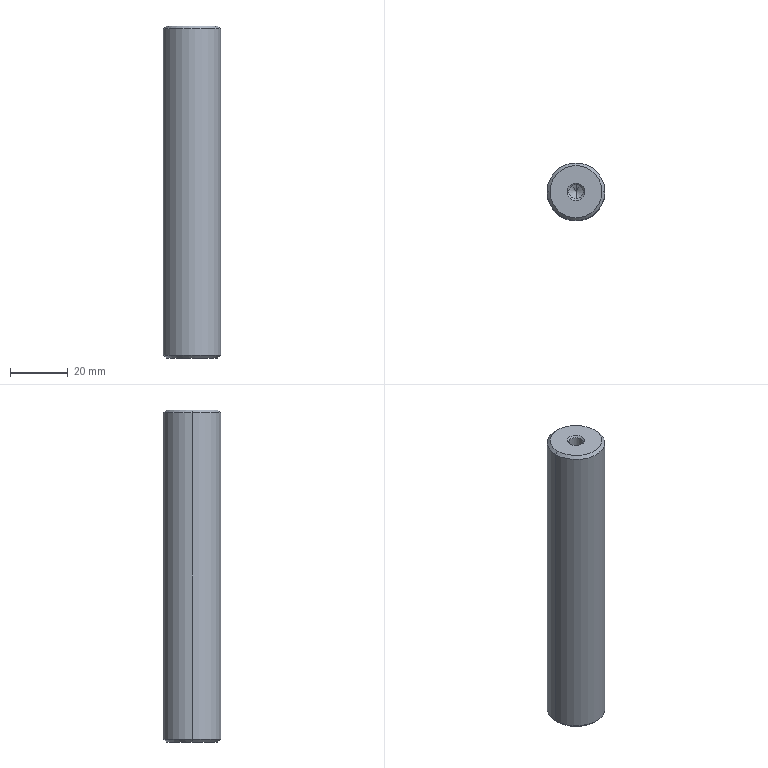Part | STEP file | 001-011-SCD21-D20-L115-M6 | 1 solid | 14 faces | box 20 x 20 x 115 mm | volume 35828 mm3 | cone 8 | cylinder 4 | plane 2 | commonest cylinder face diameters 4.917 x2 20 x2
STEP:
#1=CARTESIAN_POINT('',(0.,0.,0.));
#2=DIRECTION('',(0.,0.,1.));
#3=DIRECTION('',(1.,0.,0.));
#4=AXIS2_PLACEMENT_3D('',#1,#2,#3);
#5=CARTESIAN_POINT('',(0.,-2.458,-12.));
#6=VERTEX_POINT('',#5);
#7=CARTESIAN_POINT('',(0.,2.458,-12.));
#8=VERTEX_POINT('',#7);
#9=CARTESIAN_POINT('',(0.,0.,-12.));
#10=DIRECTION('',(0.,0.,-1.));
#11=DIRECTION('',(0.,1.,0.));
#12=AXIS2_PLACEMENT_3D('',#9,#10,#11);
#13=CIRCLE('',#12,2.458);
#14=CARTESIAN_POINT('',(0.,0.,-12.));
#15=DIRECTION('',(0.,0.,1.));
#16=DIRECTION('',(0.,-1.,0.));
#17=AXIS2_PLACEMENT_3D('',#14,#15,#16);
#18=CONICAL_SURFACE('',#17,2.458,1.047);
#19=CARTESIAN_POINT('',(9.425,0.));
#20=DIRECTION('',(-1.,0.));
#21=VECTOR('',#20,1.);
#22=LINE('',#19,#21);
#23=(GEOMETRIC_REPRESENTATION_CONTEXT(2)PARAMETRIC_REPRESENTATION_CONTEXT()REPRESENTATION_CONTEXT('',''));
#24=DEFINITIONAL_REPRESENTATION('',(#22),#23);
#25=PCURVE('',#18,#24);
#26=CARTESIAN_POINT('',(0.,0.,-13.419));
#27=DIRECTION('',(0.,0.,1.));
#28=DIRECTION('',(0.,1.,0.));
#29=AXIS2_PLACEMENT_3D('',#26,#27,#28);
#30=CYLINDRICAL_SURFACE('',#29,2.458);
#31=CARTESIAN_POINT('',(6.283,1.419));
#32=DIRECTION('',(-1.,0.));
#33=VECTOR('',#32,1.);
#34=LINE('',#31,#33);
#35=(GEOMETRIC_REPRESENTATION_CONTEXT(2)PARAMETRIC_REPRESENTATION_CONTEXT()REPRESENTATION_CONTEXT('',''));
#36=DEFINITIONAL_REPRESENTATION('',(#34),#35);
#37=PCURVE('',#30,#36);
#38=SURFACE_CURVE('',#13,(#25,#37),.PCURVE_S1.);
#39=EDGE_CURVE('',#6,#8,#38,.T.);
#40=ORIENTED_EDGE('',*,*,#39,.T.);
#41=CARTESIAN_POINT('',(0.,0.,-13.419));
#42=VERTEX_POINT('',#41);
#43=CARTESIAN_POINT('',(0.,2.458,-12.));
#44=DIRECTION('',(0.,0.866,0.5));
#45=VECTOR('',#44,1.);
#46=LINE('',#43,#45);
#47=CARTESIAN_POINT('',(3.142,0.));
#48=DIRECTION('',(0.,1.));
#49=VECTOR('',#48,1.);
#50=LINE('',#47,#49);
#51=(GEOMETRIC_REPRESENTATION_CONTEXT(2)PARAMETRIC_REPRESENTATION_CONTEXT()REPRESENTATION_CONTEXT('',''));
#52=DEFINITIONAL_REPRESENTATION('',(#50),#51);
#53=PCURVE('',#18,#52);
#54=CARTESIAN_POINT('',(0.,0.,-12.));
#55=DIRECTION('',(0.,0.,1.));
#56=DIRECTION('',(0.,-1.,0.));
#57=AXIS2_PLACEMENT_3D('',#54,#55,#56);
#58=CONICAL_SURFACE('',#57,2.458,1.047);
#59=CARTESIAN_POINT('',(3.142,0.));
#60=DIRECTION('',(0.,1.));
#61=VECTOR('',#60,1.);
#62=LINE('',#59,#61);
#63=(GEOMETRIC_REPRESENTATION_CONTEXT(2)PARAMETRIC_REPRESENTATION_CONTEXT()REPRESENTATION_CONTEXT('',''));
#64=DEFINITIONAL_REPRESENTATION('',(#62),#63);
#65=PCURVE('',#58,#64);
#66=SURFACE_CURVE('',#46,(#53,#65),.PCURVE_S1.);
#67=EDGE_CURVE('',#42,#8,#66,.T.);
#68=ORIENTED_EDGE('',*,*,#67,.F.);
#69=CARTESIAN_POINT('',(0.,-2.458,-12.));
#70=DIRECTION('',(0.,-0.866,0.5));
#71=VECTOR('',#70,1.);
#72=LINE('',#69,#71);
#73=CARTESIAN_POINT('',(6.283,0.));
#74=DIRECTION('',(0.,1.));
#75=VECTOR('',#74,1.);
#76=LINE('',#73,#75);
#77=(GEOMETRIC_REPRESENTATION_CONTEXT(2)PARAMETRIC_REPRESENTATION_CONTEXT()REPRESENTATION_CONTEXT('',''));
#78=DEFINITIONAL_REPRESENTATION('',(#76),#77);
#79=PCURVE('',#18,#78);
#80=CARTESIAN_POINT('',(0.,0.));
#81=DIRECTION('',(0.,1.));
#82=VECTOR('',#81,1.);
#83=LINE('',#80,#82);
#84=(GEOMETRIC_REPRESENTATION_CONTEXT(2)PARAMETRIC_REPRESENTATION_CONTEXT()REPRESENTATION_CONTEXT('',''));
#85=DEFINITIONAL_REPRESENTATION('',(#83),#84);
#86=PCURVE('',#58,#85);
#87=SURFACE_CURVE('',#72,(#79,#86),.PCURVE_S1.);
#88=EDGE_CURVE('',#42,#6,#87,.T.);
#89=ORIENTED_EDGE('',*,*,#88,.T.);
#90=EDGE_LOOP('',(#40,#68,#89));
#91=FACE_BOUND('',#90,.F.);
#92=ADVANCED_FACE('',(#91),#18,.F.);
#93=CARTESIAN_POINT('',(-9.,0.,0.));
#94=VERTEX_POINT('',#93);
#95=CARTESIAN_POINT('',(9.,0.,0.));
#96=VERTEX_POINT('',#95);
#97=CARTESIAN_POINT('',(0.,0.,0.));
#98=DIRECTION('',(0.,0.,-1.));
#99=DIRECTION('',(-1.,0.,0.));
#100=AXIS2_PLACEMENT_3D('',#97,#98,#99);
#101=CIRCLE('',#100,9.);
#102=CARTESIAN_POINT('',(0.,0.,0.));
#103=DIRECTION('',(0.,0.,-1.));
#104=DIRECTION('',(-1.,0.,0.));
#105=AXIS2_PLACEMENT_3D('',#102,#103,#104);
#106=CONICAL_SURFACE('',#105,9.,0.7854);
#107=CARTESIAN_POINT('',(0.,0.));
#108=DIRECTION('',(1.,0.));
#109=VECTOR('',#108,1.);
#110=LINE('',#107,#109);
#111=(GEOMETRIC_REPRESENTATION_CONTEXT(2)PARAMETRIC_REPRESENTATION_CONTEXT()REPRESENTATION_CONTEXT('',''));
#112=DEFINITIONAL_REPRESENTATION('',(#110),#111);
#113=PCURVE('',#106,#112);
#114=CARTESIAN_POINT('',(0.,0.,0.));
#115=DIRECTION('',(0.,0.,-1.));
#116=DIRECTION('',(0.,-1.,0.));
#117=AXIS2_PLACEMENT_3D('',#114,#115,#116);
#118=PLANE('',#117);
#119=CARTESIAN_POINT('',(0.,0.));
#120=DIRECTION('',(0.,1.));
#121=AXIS2_PLACEMENT_2D('',#119,#120);
#122=CIRCLE('',#121,9.);
#123=(GEOMETRIC_REPRESENTATION_CONTEXT(2)PARAMETRIC_REPRESENTATION_CONTEXT()REPRESENTATION_CONTEXT('',''));
#124=DEFINITIONAL_REPRESENTATION('',(#122),#123);
#125=PCURVE('',#118,#124);
#126=SURFACE_CURVE('',#101,(#113,#125),.PCURVE_S1.);
#127=EDGE_CURVE('',#94,#96,#126,.T.);
#128=ORIENTED_EDGE('',*,*,#127,.T.);
#129=CARTESIAN_POINT('',(10.,0.,-1.));
#130=VERTEX_POINT('',#129);
#131=CARTESIAN_POINT('',(9.,0.,0.));
#132=DIRECTION('',(0.7071,0.,-0.7071));
#133=VECTOR('',#132,1.);
#134=LINE('',#131,#133);
#135=CARTESIAN_POINT('',(3.142,0.));
#136=DIRECTION('',(0.,1.));
#137=VECTOR('',#136,1.);
#138=LINE('',#135,#137);
#139=(GEOMETRIC_REPRESENTATION_CONTEXT(2)PARAMETRIC_REPRESENTATION_CONTEXT()REPRESENTATION_CONTEXT('',''));
#140=DEFINITIONAL_REPRESENTATION('',(#138),#139);
#141=PCURVE('',#106,#140);
#142=CARTESIAN_POINT('',(0.,0.,0.));
#143=DIRECTION('',(0.,0.,-1.));
#144=DIRECTION('',(-1.,0.,0.));
#145=AXIS2_PLACEMENT_3D('',#142,#143,#144);
#146=CONICAL_SURFACE('',#145,9.,0.7854);
#147=CARTESIAN_POINT('',(3.142,0.));
#148=DIRECTION('',(0.,1.));
#149=VECTOR('',#148,1.);
#150=LINE('',#147,#149);
#151=(GEOMETRIC_REPRESENTATION_CONTEXT(2)PARAMETRIC_REPRESENTATION_CONTEXT()REPRESENTATION_CONTEXT('',''));
#152=DEFINITIONAL_REPRESENTATION('',(#150),#151);
#153=PCURVE('',#146,#152);
#154=SURFACE_CURVE('',#134,(#141,#153),.PCURVE_S1.);
#155=EDGE_CURVE('',#96,#130,#154,.T.);
#156=ORIENTED_EDGE('',*,*,#155,.T.);
#157=CARTESIAN_POINT('',(-10.,0.,-1.));
#158=VERTEX_POINT('',#157);
#159=CARTESIAN_POINT('',(0.,0.,-1.));
#160=DIRECTION('',(0.,0.,-1.));
#161=DIRECTION('',(-1.,0.,0.));
#162=AXIS2_PLACEMENT_3D('',#159,#160,#161);
#163=CIRCLE('',#162,10.);
#164=CARTESIAN_POINT('',(0.,1.));
#165=DIRECTION('',(1.,0.));
#166=VECTOR('',#165,1.);
#167=LINE('',#164,#166);
#168=(GEOMETRIC_REPRESENTATION_CONTEXT(2)PARAMETRIC_REPRESENTATION_CONTEXT()REPRESENTATION_CONTEXT('',''));
#169=DEFINITIONAL_REPRESENTATION('',(#167),#168);
#170=PCURVE('',#106,#169);
#171=CARTESIAN_POINT('',(0.,0.,-115.));
#172=DIRECTION('',(0.,0.,1.));
#173=DIRECTION('',(-1.,0.,0.));
#174=AXIS2_PLACEMENT_3D('',#171,#172,#173);
#175=CYLINDRICAL_SURFACE('',#174,10.);
#176=CARTESIAN_POINT('',(6.283,114.));
#177=DIRECTION('',(-1.,0.));
#178=VECTOR('',#177,1.);
#179=LINE('',#176,#178);
#180=(GEOMETRIC_REPRESENTATION_CONTEXT(2)PARAMETRIC_REPRESENTATION_CONTEXT()REPRESENTATION_CONTEXT('',''));
#181=DEFINITIONAL_REPRESENTATION('',(#179),#180);
#182=PCURVE('',#175,#181);
#183=SURFACE_CURVE('',#163,(#170,#182),.PCURVE_S1.);
#184=EDGE_CURVE('',#158,#130,#183,.T.);
#185=ORIENTED_EDGE('',*,*,#184,.F.);
#186=CARTESIAN_POINT('',(-9.,0.,0.));
#187=DIRECTION('',(-0.7071,0.,-0.7071));
#188=VECTOR('',#187,1.);
#189=LINE('',#186,#188);
#190=CARTESIAN_POINT('',(0.,0.));
#191=DIRECTION('',(0.,1.));
#192=VECTOR('',#191,1.);
#193=LINE('',#190,#192);
#194=(GEOMETRIC_REPRESENTATION_CONTEXT(2)PARAMETRIC_REPRESENTATION_CONTEXT()REPRESENTATION_CONTEXT('',''));
#195=DEFINITIONAL_REPRESENTATION('',(#193),#194);
#196=PCURVE('',#106,#195);
#197=CARTESIAN_POINT('',(6.283,0.));
#198=DIRECTION('',(0.,1.));
#199=VECTOR('',#198,1.);
#200=LINE('',#197,#199);
#201=(GEOMETRIC_REPRESENTATION_CONTEXT(2)PARAMETRIC_REPRESENTATION_CONTEXT()REPRESENTATION_CONTEXT('',''));
#202=DEFINITIONAL_REPRESENTATION('',(#200),#201);
#203=PCURVE('',#146,#202);
#204=SURFACE_CURVE('',#189,(#196,#203),.PCURVE_S1.);
#205=EDGE_CURVE('',#94,#158,#204,.T.);
#206=ORIENTED_EDGE('',*,*,#205,.F.);
#207=EDGE_LOOP('',(#128,#156,#185,#206));
#208=FACE_BOUND('',#207,.T.);
#209=ADVANCED_FACE('',(#208),#106,.T.);
#210=CARTESIAN_POINT('',(0.,-2.458,-0.5415));
#211=VERTEX_POINT('',#210);
#212=CARTESIAN_POINT('',(0.,-3.,0.));
#213=VERTEX_POINT('',#212);
#214=CARTESIAN_POINT('',(0.,-3.,0.));
#215=DIRECTION('',(0.,-0.7071,0.7071));
#216=VECTOR('',#215,1.);
#217=LINE('',#214,#216);
#218=CARTESIAN_POINT('',(0.,0.,0.));
#219=DIRECTION('',(0.,0.,1.));
#220=DIRECTION('',(0.,-1.,0.));
#221=AXIS2_PLACEMENT_3D('',#218,#219,#220);
#222=CONICAL_SURFACE('',#221,3.,0.7854);
#223=CARTESIAN_POINT('',(6.283,0.));
#224=DIRECTION('',(0.,1.));
#225=VECTOR('',#224,1.);
#226=LINE('',#223,#225);
#227=(GEOMETRIC_REPRESENTATION_CONTEXT(2)PARAMETRIC_REPRESENTATION_CONTEXT()REPRESENTATION_CONTEXT('',''));
#228=DEFINITIONAL_REPRESENTATION('',(#226),#227);
#229=PCURVE('',#222,#228);
#230=CARTESIAN_POINT('',(0.,0.,0.));
#231=DIRECTION('',(0.,0.,1.));
#232=DIRECTION('',(0.,-1.,0.));
#233=AXIS2_PLACEMENT_3D('',#230,#231,#232);
#234=CONICAL_SURFACE('',#233,3.,0.7854);
#235=CARTESIAN_POINT('',(0.,0.));
#236=DIRECTION('',(0.,1.));
#237=VECTOR('',#236,1.);
#238=LINE('',#235,#237);
#239=(GEOMETRIC_REPRESENTATION_CONTEXT(2)PARAMETRIC_REPRESENTATION_CONTEXT()REPRESENTATION_CONTEXT('',''));
#240=DEFINITIONAL_REPRESENTATION('',(#238),#239);
#241=PCURVE('',#234,#240);
#242=SURFACE_CURVE('',#217,(#229,#241),.PCURVE_S1.);
#243=EDGE_CURVE('',#211,#213,#242,.T.);
#244=ORIENTED_EDGE('',*,*,#243,.T.);
#245=CARTESIAN_POINT('',(0.,3.,0.));
#246=VERTEX_POINT('',#245);
#247=CARTESIAN_POINT('',(0.,0.,0.));
#248=DIRECTION('',(0.,0.,-1.));
#249=DIRECTION('',(0.,1.,0.));
#250=AXIS2_PLACEMENT_3D('',#247,#248,#249);
#251=CIRCLE('',#250,3.);
#252=CARTESIAN_POINT('',(9.425,0.));
#253=DIRECTION('',(-1.,0.));
#254=VECTOR('',#253,1.);
#255=LINE('',#252,#254);
#256=(GEOMETRIC_REPRESENTATION_CONTEXT(2)PARAMETRIC_REPRESENTATION_CONTEXT()REPRESENTATION_CONTEXT('',''));
#257=DEFINITIONAL_REPRESENTATION('',(#255),#256);
#258=PCURVE('',#222,#257);
#259=CARTESIAN_POINT('',(0.,0.));
#260=DIRECTION('',(-1.,0.));
#261=AXIS2_PLACEMENT_2D('',#259,#260);
#262=CIRCLE('',#261,3.);
#263=(GEOMETRIC_REPRESENTATION_CONTEXT(2)PARAMETRIC_REPRESENTATION_CONTEXT()REPRESENTATION_CONTEXT('',''));
#264=DEFINITIONAL_REPRESENTATION('',(#262),#263);
#265=PCURVE('',#118,#264);
#266=SURFACE_CURVE('',#251,(#258,#265),.PCURVE_S1.);
#267=EDGE_CURVE('',#213,#246,#266,.T.);
#268=ORIENTED_EDGE('',*,*,#267,.T.);
#269=CARTESIAN_POINT('',(0.,2.458,-0.5415));
#270=VERTEX_POINT('',#269);
#271=CARTESIAN_POINT('',(0.,3.,0.));
#272=DIRECTION('',(0.,0.7071,0.7071));
#273=VECTOR('',#272,1.);
#274=LINE('',#271,#273);
#275=CARTESIAN_POINT('',(3.142,0.));
#276=DIRECTION('',(0.,1.));
#277=VECTOR('',#276,1.);
#278=LINE('',#275,#277);
#279=(GEOMETRIC_REPRESENTATION_CONTEXT(2)PARAMETRIC_REPRESENTATION_CONTEXT()REPRESENTATION_CONTEXT('',''));
#280=DEFINITIONAL_REPRESENTATION('',(#278),#279);
#281=PCURVE('',#222,#280);
#282=CARTESIAN_POINT('',(3.142,0.));
#283=DIRECTION('',(0.,1.));
#284=VECTOR('',#283,1.);
#285=LINE('',#282,#284);
#286=(GEOMETRIC_REPRESENTATION_CONTEXT(2)PARAMETRIC_REPRESENTATION_CONTEXT()REPRESENTATION_CONTEXT('',''));
#287=DEFINITIONAL_REPRESENTATION('',(#285),#286);
#288=PCURVE('',#234,#287);
#289=SURFACE_CURVE('',#274,(#281,#288),.PCURVE_S1.);
#290=EDGE_CURVE('',#270,#246,#289,.T.);
#291=ORIENTED_EDGE('',*,*,#290,.F.);
#292=CARTESIAN_POINT('',(0.,0.,-0.5415));
#293=DIRECTION('',(0.,0.,-1.));
#294=DIRECTION('',(0.,1.,0.));
#295=AXIS2_PLACEMENT_3D('',#292,#293,#294);
#296=CIRCLE('',#295,2.458);
#297=CARTESIAN_POINT('',(9.425,-0.5415));
#298=DIRECTION('',(-1.,0.));
#299=VECTOR('',#298,1.);
#300=LINE('',#297,#299);
#301=(GEOMETRIC_REPRESENTATION_CONTEXT(2)PARAMETRIC_REPRESENTATION_CONTEXT()REPRESENTATION_CONTEXT('',''));
#302=DEFINITIONAL_REPRESENTATION('',(#300),#301);
#303=PCURVE('',#222,#302);
#304=CARTESIAN_POINT('',(6.283,12.878));
#305=DIRECTION('',(-1.,0.));
#306=VECTOR('',#305,1.);
#307=LINE('',#304,#306);
#308=(GEOMETRIC_REPRESENTATION_CONTEXT(2)PARAMETRIC_REPRESENTATION_CONTEXT()REPRESENTATION_CONTEXT('',''));
#309=DEFINITIONAL_REPRESENTATION('',(#307),#308);
#310=PCURVE('',#30,#309);
#311=SURFACE_CURVE('',#296,(#303,#310),.PCURVE_S1.);
#312=EDGE_CURVE('',#211,#270,#311,.T.);
#313=ORIENTED_EDGE('',*,*,#312,.F.);
#314=EDGE_LOOP('',(#244,#268,#291,#313));
#315=FACE_BOUND('',#314,.F.);
#316=ADVANCED_FACE('',(#315),#222,.F.);
#317=CARTESIAN_POINT('',(0.,2.458,-13.419));
#318=DIRECTION('',(0.,0.,1.));
#319=VECTOR('',#318,1.);
#320=LINE('',#317,#319);
#321=CARTESIAN_POINT('',(0.,0.,-13.419));
#322=DIRECTION('',(0.,0.,1.));
#323=DIRECTION('',(0.,1.,0.));
#324=AXIS2_PLACEMENT_3D('',#321,#322,#323);
#325=CYLINDRICAL_SURFACE('',#324,2.458);
#326=CARTESIAN_POINT('',(6.283,0.));
#327=DIRECTION('',(0.,1.));
#328=VECTOR('',#327,1.);
#329=LINE('',#326,#328);
#330=(GEOMETRIC_REPRESENTATION_CONTEXT(2)PARAMETRIC_REPRESENTATION_CONTEXT()REPRESENTATION_CONTEXT('',''));
#331=DEFINITIONAL_REPRESENTATION('',(#329),#330);
#332=PCURVE('',#325,#331);
#333=CARTESIAN_POINT('',(0.,0.));
#334=DIRECTION('',(0.,1.));
#335=VECTOR('',#334,1.);
#336=LINE('',#333,#335);
#337=(GEOMETRIC_REPRESENTATION_CONTEXT(2)PARAMETRIC_REPRESENTATION_CONTEXT()REPRESENTATION_CONTEXT('',''));
#338=DEFINITIONAL_REPRESENTATION('',(#336),#337);
#339=PCURVE('',#30,#338);
#340=SURFACE_CURVE('',#320,(#332,#339),.PCURVE_S1.);
#341=EDGE_CURVE('',#8,#270,#340,.T.);
#342=ORIENTED_EDGE('',*,*,#341,.T.);
#343=CARTESIAN_POINT('',(0.,0.,-0.5415));
#344=DIRECTION('',(0.,0.,-1.));
#345=DIRECTION('',(0.,1.,0.));
#346=AXIS2_PLACEMENT_3D('',#343,#344,#345);
#347=CIRCLE('',#346,2.458);
#348=CARTESIAN_POINT('',(6.283,12.878));
#349=DIRECTION('',(-1.,0.));
#350=VECTOR('',#349,1.);
#351=LINE('',#348,#350);
#352=(GEOMETRIC_REPRESENTATION_CONTEXT(2)PARAMETRIC_REPRESENTATION_CONTEXT()REPRESENTATION_CONTEXT('',''));
#353=DEFINITIONAL_REPRESENTATION('',(#351),#352);
#354=PCURVE('',#325,#353);
#355=CARTESIAN_POINT('',(3.142,-0.5415));
#356=DIRECTION('',(-1.,0.));
#357=VECTOR('',#356,1.);
#358=LINE('',#355,#357);
#359=(GEOMETRIC_REPRESENTATION_CONTEXT(2)PARAMETRIC_REPRESENTATION_CONTEXT()REPRESENTATION_CONTEXT('',''));
#360=DEFINITIONAL_REPRESENTATION('',(#358),#359);
#361=PCURVE('',#234,#360);
#362=SURFACE_CURVE('',#347,(#354,#361),.PCURVE_S1.);
#363=EDGE_CURVE('',#270,#211,#362,.T.);
#364=ORIENTED_EDGE('',*,*,#363,.T.);
#365=CARTESIAN_POINT('',(0.,-2.458,-13.419));
#366=DIRECTION('',(0.,0.,1.));
#367=VECTOR('',#366,1.);
#368=LINE('',#365,#367);
#369=CARTESIAN_POINT('',(3.142,0.));
#370=DIRECTION('',(0.,1.));
#371=VECTOR('',#370,1.);
#372=LINE('',#369,#371);
#373=(GEOMETRIC_REPRESENTATION_CONTEXT(2)PARAMETRIC_REPRESENTATION_CONTEXT()REPRESENTATION_CONTEXT('',''));
#374=DEFINITIONAL_REPRESENTATION('',(#372),#373);
#375=PCURVE('',#325,#374);
#376=CARTESIAN_POINT('',(3.142,0.));
#377=DIRECTION('',(0.,1.));
#378=VECTOR('',#377,1.);
#379=LINE('',#376,#378);
#380=(GEOMETRIC_REPRESENTATION_CONTEXT(2)PARAMETRIC_REPRESENTATION_CONTEXT()REPRESENTATION_CONTEXT('',''));
#381=DEFINITIONAL_REPRESENTATION('',(#379),#380);
#382=PCURVE('',#30,#381);
#383=SURFACE_CURVE('',#368,(#375,#382),.PCURVE_S1.);
#384=EDGE_CURVE('',#6,#211,#383,.T.);
#385=ORIENTED_EDGE('',*,*,#384,.F.);
#386=CARTESIAN_POINT('',(0.,0.,-12.));
#387=DIRECTION('',(0.,0.,-1.));
#388=DIRECTION('',(0.,1.,0.));
#389=AXIS2_PLACEMENT_3D('',#386,#387,#388);
#390=CIRCLE('',#389,2.458);
#391=CARTESIAN_POINT('',(6.283,1.419));
#392=DIRECTION('',(-1.,0.));
#393=VECTOR('',#392,1.);
#394=LINE('',#391,#393);
#395=(GEOMETRIC_REPRESENTATION_CONTEXT(2)PARAMETRIC_REPRESENTATION_CONTEXT()REPRESENTATION_CONTEXT('',''));
#396=DEFINITIONAL_REPRESENTATION('',(#394),#395);
#397=PCURVE('',#325,#396);
#398=CARTESIAN_POINT('',(3.142,0.));
#399=DIRECTION('',(-1.,0.));
#400=VECTOR('',#399,1.);
#401=LINE('',#398,#400);
#402=(GEOMETRIC_REPRESENTATION_CONTEXT(2)PARAMETRIC_REPRESENTATION_CONTEXT()REPRESENTATION_CONTEXT('',''));
#403=DEFINITIONAL_REPRESENTATION('',(#401),#402);
#404=PCURVE('',#58,#403);
#405=SURFACE_CURVE('',#390,(#397,#404),.PCURVE_S1.);
#406=EDGE_CURVE('',#8,#6,#405,.T.);
#407=ORIENTED_EDGE('',*,*,#406,.F.);
#408=EDGE_LOOP('',(#342,#364,#385,#407));
#409=FACE_BOUND('',#408,.F.);
#410=ADVANCED_FACE('',(#409),#325,.F.);
#411=CARTESIAN_POINT('',(-9.,0.,-115.));
#412=VERTEX_POINT('',#411);
#413=CARTESIAN_POINT('',(9.,0.,-115.));
#414=VERTEX_POINT('',#413);
#415=CARTESIAN_POINT('',(0.,0.,-115.));
#416=DIRECTION('',(0.,0.,-1.));
#417=DIRECTION('',(-1.,0.,0.));
#418=AXIS2_PLACEMENT_3D('',#415,#416,#417);
#419=CIRCLE('',#418,9.);
#420=CARTESIAN_POINT('',(0.,0.,-114.));
#421=DIRECTION('',(0.,0.,1.));
#422=DIRECTION('',(1.,0.,0.));
#423=AXIS2_PLACEMENT_3D('',#420,#421,#422);
#424=CONICAL_SURFACE('',#423,10.,0.7854);
#425=CARTESIAN_POINT('',(3.142,-1.));
#426=DIRECTION('',(-1.,0.));
#427=VECTOR('',#426,1.);
#428=LINE('',#425,#427);
#429=(GEOMETRIC_REPRESENTATION_CONTEXT(2)PARAMETRIC_REPRESENTATION_CONTEXT()REPRESENTATION_CONTEXT('',''));
#430=DEFINITIONAL_REPRESENTATION('',(#428),#429);
#431=PCURVE('',#424,#430);
#432=CARTESIAN_POINT('',(0.,9.,-115.));
#433=DIRECTION('',(0.,0.,1.));
#434=DIRECTION('',(1.,0.,0.));
#435=AXIS2_PLACEMENT_3D('',#432,#433,#434);
#436=PLANE('',#435);
#437=CARTESIAN_POINT('',(-9.,-9.));
#438=CARTESIAN_POINT('',(-9.,6.588));
#439=CARTESIAN_POINT('',(4.5,-1.206));
#440=CARTESIAN_POINT('',(18.,-9.));
#441=CARTESIAN_POINT('',(4.5,-16.794));
#442=CARTESIAN_POINT('',(-9.,-24.588));
#443=CARTESIAN_POINT('',(-9.,-9.));
#444=(BOUNDED_CURVE()B_SPLINE_CURVE(2,(#437,#438,#439,#440,#441,#442,#443),.UNSPECIFIED.,.T.,.F.)B_SPLINE_CURVE_WITH_KNOTS((1,2,2,2,2,1),(-2.094,0.,2.094,4.189,6.283,8.378),.UNSPECIFIED.)CURVE()GEOMETRIC_REPRESENTATION_ITEM()RATIONAL_B_SPLINE_CURVE((1.,0.5,1.,0.5,1.,0.5,1.))REPRESENTATION_ITEM(''));
#445=(GEOMETRIC_REPRESENTATION_CONTEXT(2)PARAMETRIC_REPRESENTATION_CONTEXT()REPRESENTATION_CONTEXT('',''));
#446=DEFINITIONAL_REPRESENTATION('',(#444),#445);
#447=PCURVE('',#436,#446);
#448=SURFACE_CURVE('',#419,(#431,#447),.PCURVE_S1.);
#449=EDGE_CURVE('',#412,#414,#448,.T.);
#450=ORIENTED_EDGE('',*,*,#449,.F.);
#451=CARTESIAN_POINT('',(-10.,0.,-114.));
#452=VERTEX_POINT('',#451);
#453=CARTESIAN_POINT('',(-10.,0.,-114.));
#454=DIRECTION('',(-0.7071,0.,0.7071));
#455=VECTOR('',#454,1.);
#456=LINE('',#453,#455);
#457=CARTESIAN_POINT('',(3.142,0.));
#458=DIRECTION('',(0.,1.));
#459=VECTOR('',#458,1.);
#460=LINE('',#457,#459);
#461=(GEOMETRIC_REPRESENTATION_CONTEXT(2)PARAMETRIC_REPRESENTATION_CONTEXT()REPRESENTATION_CONTEXT('',''));
#462=DEFINITIONAL_REPRESENTATION('',(#460),#461);
#463=PCURVE('',#424,#462);
#464=CARTESIAN_POINT('',(0.,0.,-114.));
#465=DIRECTION('',(0.,0.,1.));
#466=DIRECTION('',(1.,0.,0.));
#467=AXIS2_PLACEMENT_3D('',#464,#465,#466);
#468=CONICAL_SURFACE('',#467,10.,0.7854);
#469=CARTESIAN_POINT('',(3.142,0.));
#470=DIRECTION('',(0.,1.));
#471=VECTOR('',#470,1.);
#472=LINE('',#469,#471);
#473=(GEOMETRIC_REPRESENTATION_CONTEXT(2)PARAMETRIC_REPRESENTATION_CONTEXT()REPRESENTATION_CONTEXT('',''));
#474=DEFINITIONAL_REPRESENTATION('',(#472),#473);
#475=PCURVE('',#468,#474);
#476=SURFACE_CURVE('',#456,(#463,#475),.PCURVE_S1.);
#477=EDGE_CURVE('',#412,#452,#476,.T.);
#478=ORIENTED_EDGE('',*,*,#477,.T.);
#479=CARTESIAN_POINT('',(10.,0.,-114.));
#480=VERTEX_POINT('',#479);
#481=CARTESIAN_POINT('',(0.,0.,-114.));
#482=DIRECTION('',(0.,0.,-1.));
#483=DIRECTION('',(-1.,0.,0.));
#484=AXIS2_PLACEMENT_3D('',#481,#482,#483);
#485=CIRCLE('',#484,10.);
#486=CARTESIAN_POINT('',(3.142,0.));
#487=DIRECTION('',(-1.,0.));
#488=VECTOR('',#487,1.);
#489=LINE('',#486,#488);
#490=(GEOMETRIC_REPRESENTATION_CONTEXT(2)PARAMETRIC_REPRESENTATION_CONTEXT()REPRESENTATION_CONTEXT('',''));
#491=DEFINITIONAL_REPRESENTATION('',(#489),#490);
#492=PCURVE('',#424,#491);
#493=CARTESIAN_POINT('',(6.283,1.));
#494=DIRECTION('',(-1.,0.));
#495=VECTOR('',#494,1.);
#496=LINE('',#493,#495);
#497=(GEOMETRIC_REPRESENTATION_CONTEXT(2)PARAMETRIC_REPRESENTATION_CONTEXT()REPRESENTATION_CONTEXT('',''));
#498=DEFINITIONAL_REPRESENTATION('',(#496),#497);
#499=PCURVE('',#175,#498);
#500=SURFACE_CURVE('',#485,(#492,#499),.PCURVE_S1.);
#501=EDGE_CURVE('',#452,#480,#500,.T.);
#502=ORIENTED_EDGE('',*,*,#501,.T.);
#503=CARTESIAN_POINT('',(10.,0.,-114.));
#504=DIRECTION('',(0.7071,0.,0.7071));
#505=VECTOR('',#504,1.);
#506=LINE('',#503,#505);
#507=CARTESIAN_POINT('',(0.,0.));
#508=DIRECTION('',(0.,1.));
#509=VECTOR('',#508,1.);
#510=LINE('',#507,#509);
#511=(GEOMETRIC_REPRESENTATION_CONTEXT(2)PARAMETRIC_REPRESENTATION_CONTEXT()REPRESENTATION_CONTEXT('',''));
#512=DEFINITIONAL_REPRESENTATION('',(#510),#511);
#513=PCURVE('',#424,#512);
#514=CARTESIAN_POINT('',(6.283,0.));
#515=DIRECTION('',(0.,1.));
#516=VECTOR('',#515,1.);
#517=LINE('',#514,#516);
#518=(GEOMETRIC_REPRESENTATION_CONTEXT(2)PARAMETRIC_REPRESENTATION_CONTEXT()REPRESENTATION_CONTEXT('',''));
#519=DEFINITIONAL_REPRESENTATION('',(#517),#518);
#520=PCURVE('',#468,#519);
#521=SURFACE_CURVE('',#506,(#513,#520),.PCURVE_S1.);
#522=EDGE_CURVE('',#414,#480,#521,.T.);
#523=ORIENTED_EDGE('',*,*,#522,.F.);
#524=EDGE_LOOP('',(#450,#478,#502,#523));
#525=FACE_BOUND('',#524,.T.);
#526=ADVANCED_FACE('',(#525),#424,.T.);
#527=CARTESIAN_POINT('',(0.,0.,-114.));
#528=DIRECTION('',(0.,0.,-1.));
#529=DIRECTION('',(-1.,0.,0.));
#530=AXIS2_PLACEMENT_3D('',#527,#528,#529);
#531=CIRCLE('',#530,10.);
#532=CARTESIAN_POINT('',(0.,0.,-115.));
#533=DIRECTION('',(0.,0.,1.));
#534=DIRECTION('',(-1.,0.,0.));
#535=AXIS2_PLACEMENT_3D('',#532,#533,#534);
#536=CYLINDRICAL_SURFACE('',#535,10.);
#537=CARTESIAN_POINT('',(6.283,1.));
#538=DIRECTION('',(-1.,0.));
#539=VECTOR('',#538,1.);
#540=LINE('',#537,#539);
#541=(GEOMETRIC_REPRESENTATION_CONTEXT(2)PARAMETRIC_REPRESENTATION_CONTEXT()REPRESENTATION_CONTEXT('',''));
#542=DEFINITIONAL_REPRESENTATION('',(#540),#541);
#543=PCURVE('',#536,#542);
#544=CARTESIAN_POINT('',(9.425,0.));
#545=DIRECTION('',(-1.,0.));
#546=VECTOR('',#545,1.);
#547=LINE('',#544,#546);
#548=(GEOMETRIC_REPRESENTATION_CONTEXT(2)PARAMETRIC_REPRESENTATION_CONTEXT()REPRESENTATION_CONTEXT('',''));
#549=DEFINITIONAL_REPRESENTATION('',(#547),#548);
#550=PCURVE('',#468,#549);
#551=SURFACE_CURVE('',#531,(#543,#550),.PCURVE_S1.);
#552=EDGE_CURVE('',#480,#452,#551,.T.);
#553=ORIENTED_EDGE('',*,*,#552,.F.);
#554=CARTESIAN_POINT('',(10.,0.,-115.));
#555=DIRECTION('',(0.,0.,1.));
#556=VECTOR('',#555,1.);
#557=LINE('',#554,#556);
#558=CARTESIAN_POINT('',(3.142,0.));
#559=DIRECTION('',(0.,1.));
#560=VECTOR('',#559,1.);
#561=LINE('',#558,#560);
#562=(GEOMETRIC_REPRESENTATION_CONTEXT(2)PARAMETRIC_REPRESENTATION_CONTEXT()REPRESENTATION_CONTEXT('',''));
#563=DEFINITIONAL_REPRESENTATION('',(#561),#562);
#564=PCURVE('',#536,#563);
#565=CARTESIAN_POINT('',(3.142,0.));
#566=DIRECTION('',(0.,1.));
#567=VECTOR('',#566,1.);
#568=LINE('',#565,#567);
#569=(GEOMETRIC_REPRESENTATION_CONTEXT(2)PARAMETRIC_REPRESENTATION_CONTEXT()REPRESENTATION_CONTEXT('',''));
#570=DEFINITIONAL_REPRESENTATION('',(#568),#569);
#571=PCURVE('',#175,#570);
#572=SURFACE_CURVE('',#557,(#564,#571),.PCURVE_S1.);
#573=EDGE_CURVE('',#480,#130,#572,.T.);
#574=ORIENTED_EDGE('',*,*,#573,.T.);
#575=CARTESIAN_POINT('',(0.,0.,-1.));
#576=DIRECTION('',(0.,0.,-1.));
#577=DIRECTION('',(-1.,0.,0.));
#578=AXIS2_PLACEMENT_3D('',#575,#576,#577);
#579=CIRCLE('',#578,10.);
#580=CARTESIAN_POINT('',(6.283,114.));
#581=DIRECTION('',(-1.,0.));
#582=VECTOR('',#581,1.);
#583=LINE('',#580,#582);
#584=(GEOMETRIC_REPRESENTATION_CONTEXT(2)PARAMETRIC_REPRESENTATION_CONTEXT()REPRESENTATION_CONTEXT('',''));
#585=DEFINITIONAL_REPRESENTATION('',(#583),#584);
#586=PCURVE('',#536,#585);
#587=CARTESIAN_POINT('',(0.,1.));
#588=DIRECTION('',(1.,0.));
#589=VECTOR('',#588,1.);
#590=LINE('',#587,#589);
#591=(GEOMETRIC_REPRESENTATION_CONTEXT(2)PARAMETRIC_REPRESENTATION_CONTEXT()REPRESENTATION_CONTEXT('',''));
#592=DEFINITIONAL_REPRESENTATION('',(#590),#591);
#593=PCURVE('',#146,#592);
#594=SURFACE_CURVE('',#579,(#586,#593),.PCURVE_S1.);
#595=EDGE_CURVE('',#130,#158,#594,.T.);
#596=ORIENTED_EDGE('',*,*,#595,.T.);
#597=CARTESIAN_POINT('',(-10.,0.,-115.));
#598=DIRECTION('',(0.,0.,1.));
#599=VECTOR('',#598,1.);
#600=LINE('',#597,#599);
#601=CARTESIAN_POINT('',(0.,0.));
#602=DIRECTION('',(0.,1.));
#603=VECTOR('',#602,1.);
#604=LINE('',#601,#603);
#605=(GEOMETRIC_REPRESENTATION_CONTEXT(2)PARAMETRIC_REPRESENTATION_CONTEXT()REPRESENTATION_CONTEXT('',''));
#606=DEFINITIONAL_REPRESENTATION('',(#604),#605);
#607=PCURVE('',#536,#606);
#608=CARTESIAN_POINT('',(6.283,0.));
#609=DIRECTION('',(0.,1.));
#610=VECTOR('',#609,1.);
#611=LINE('',#608,#610);
#612=(GEOMETRIC_REPRESENTATION_CONTEXT(2)PARAMETRIC_REPRESENTATION_CONTEXT()REPRESENTATION_CONTEXT('',''));
#613=DEFINITIONAL_REPRESENTATION('',(#611),#612);
#614=PCURVE('',#175,#613);
#615=SURFACE_CURVE('',#600,(#607,#614),.PCURVE_S1.);
#616=EDGE_CURVE('',#452,#158,#615,.T.);
#617=ORIENTED_EDGE('',*,*,#616,.F.);
#618=EDGE_LOOP('',(#553,#574,#596,#617));
#619=FACE_BOUND('',#618,.T.);
#620=ADVANCED_FACE('',(#619),#536,.T.);
#621=ORIENTED_EDGE('',*,*,#573,.F.);
#622=ORIENTED_EDGE('',*,*,#501,.F.);
#623=ORIENTED_EDGE('',*,*,#616,.T.);
#624=ORIENTED_EDGE('',*,*,#184,.T.);
#625=EDGE_LOOP('',(#621,#622,#623,#624));
#626=FACE_BOUND('',#625,.T.);
#627=ADVANCED_FACE('',(#626),#175,.T.);
#628=ORIENTED_EDGE('',*,*,#477,.F.);
#629=CARTESIAN_POINT('',(0.,0.,-115.));
#630=DIRECTION('',(0.,0.,-1.));
#631=DIRECTION('',(-1.,0.,0.));
#632=AXIS2_PLACEMENT_3D('',#629,#630,#631);
#633=CIRCLE('',#632,9.);
#634=CARTESIAN_POINT('',(9.425,-1.));
#635=DIRECTION('',(-1.,0.));
#636=VECTOR('',#635,1.);
#637=LINE('',#634,#636);
#638=(GEOMETRIC_REPRESENTATION_CONTEXT(2)PARAMETRIC_REPRESENTATION_CONTEXT()REPRESENTATION_CONTEXT('',''));
#639=DEFINITIONAL_REPRESENTATION('',(#637),#638);
#640=PCURVE('',#468,#639);
#641=CARTESIAN_POINT('',(-9.,-9.));
#642=CARTESIAN_POINT('',(-9.,6.588));
#643=CARTESIAN_POINT('',(4.5,-1.206));
#644=CARTESIAN_POINT('',(18.,-9.));
#645=CARTESIAN_POINT('',(4.5,-16.794));
#646=CARTESIAN_POINT('',(-9.,-24.588));
#647=CARTESIAN_POINT('',(-9.,-9.));
#648=(BOUNDED_CURVE()B_SPLINE_CURVE(2,(#641,#642,#643,#644,#645,#646,#647),.UNSPECIFIED.,.T.,.F.)B_SPLINE_CURVE_WITH_KNOTS((1,2,2,2,2,1),(-2.094,0.,2.094,4.189,6.283,8.378),.UNSPECIFIED.)CURVE()GEOMETRIC_REPRESENTATION_ITEM()RATIONAL_B_SPLINE_CURVE((1.,0.5,1.,0.5,1.,0.5,1.))REPRESENTATION_ITEM(''));
#649=(GEOMETRIC_REPRESENTATION_CONTEXT(2)PARAMETRIC_REPRESENTATION_CONTEXT()REPRESENTATION_CONTEXT('',''));
#650=DEFINITIONAL_REPRESENTATION('',(#648),#649);
#651=PCURVE('',#436,#650);
#652=SURFACE_CURVE('',#633,(#640,#651),.PCURVE_S1.);
#653=EDGE_CURVE('',#414,#412,#652,.T.);
#654=ORIENTED_EDGE('',*,*,#653,.F.);
#655=ORIENTED_EDGE('',*,*,#522,.T.);
#656=ORIENTED_EDGE('',*,*,#552,.T.);
#657=EDGE_LOOP('',(#628,#654,#655,#656));
#658=FACE_BOUND('',#657,.T.);
#659=ADVANCED_FACE('',(#658),#468,.T.);
#660=ORIENTED_EDGE('',*,*,#653,.T.);
#661=ORIENTED_EDGE('',*,*,#449,.T.);
#662=EDGE_LOOP('',(#660,#661));
#663=FACE_BOUND('',#662,.T.);
#664=ADVANCED_FACE('',(#663),#436,.F.);
#665=ORIENTED_EDGE('',*,*,#312,.T.);
#666=ORIENTED_EDGE('',*,*,#341,.F.);
#667=ORIENTED_EDGE('',*,*,#39,.F.);
#668=ORIENTED_EDGE('',*,*,#384,.T.);
#669=EDGE_LOOP('',(#665,#666,#667,#668));
#670=FACE_BOUND('',#669,.F.);
#671=ADVANCED_FACE('',(#670),#30,.F.);
#672=CARTESIAN_POINT('',(0.,0.,0.));
#673=DIRECTION('',(0.,0.,-1.));
#674=DIRECTION('',(0.,1.,0.));
#675=AXIS2_PLACEMENT_3D('',#672,#673,#674);
#676=CIRCLE('',#675,3.);
#677=CARTESIAN_POINT('',(3.142,0.));
#678=DIRECTION('',(-1.,0.));
#679=VECTOR('',#678,1.);
#680=LINE('',#677,#679);
#681=(GEOMETRIC_REPRESENTATION_CONTEXT(2)PARAMETRIC_REPRESENTATION_CONTEXT()REPRESENTATION_CONTEXT('',''));
#682=DEFINITIONAL_REPRESENTATION('',(#680),#681);
#683=PCURVE('',#234,#682);
#684=CARTESIAN_POINT('',(0.,0.));
#685=DIRECTION('',(-1.,0.));
#686=AXIS2_PLACEMENT_2D('',#684,#685);
#687=CIRCLE('',#686,3.);
#688=(GEOMETRIC_REPRESENTATION_CONTEXT(2)PARAMETRIC_REPRESENTATION_CONTEXT()REPRESENTATION_CONTEXT('',''));
#689=DEFINITIONAL_REPRESENTATION('',(#687),#688);
#690=PCURVE('',#118,#689);
#691=SURFACE_CURVE('',#676,(#683,#690),.PCURVE_S1.);
#692=EDGE_CURVE('',#246,#213,#691,.T.);
#693=ORIENTED_EDGE('',*,*,#692,.T.);
#694=ORIENTED_EDGE('',*,*,#243,.F.);
#695=ORIENTED_EDGE('',*,*,#363,.F.);
#696=ORIENTED_EDGE('',*,*,#290,.T.);
#697=EDGE_LOOP('',(#693,#694,#695,#696));
#698=FACE_BOUND('',#697,.F.);
#699=ADVANCED_FACE('',(#698),#234,.F.);
#700=ORIENTED_EDGE('',*,*,#267,.T.);
#701=ORIENTED_EDGE('',*,*,#692,.T.);
#702=EDGE_LOOP('',(#700,#701));
#703=FACE_BOUND('',#702,.T.);
#704=ORIENTED_EDGE('',*,*,#127,.F.);
#705=CARTESIAN_POINT('',(0.,0.,0.));
#706=DIRECTION('',(0.,0.,-1.));
#707=DIRECTION('',(-1.,0.,0.));
#708=AXIS2_PLACEMENT_3D('',#705,#706,#707);
#709=CIRCLE('',#708,9.);
#710=CARTESIAN_POINT('',(0.,0.));
#711=DIRECTION('',(0.,1.));
#712=AXIS2_PLACEMENT_2D('',#710,#711);
#713=CIRCLE('',#712,9.);
#714=(GEOMETRIC_REPRESENTATION_CONTEXT(2)PARAMETRIC_REPRESENTATION_CONTEXT()REPRESENTATION_CONTEXT('',''));
#715=DEFINITIONAL_REPRESENTATION('',(#713),#714);
#716=PCURVE('',#118,#715);
#717=CARTESIAN_POINT('',(0.,0.));
#718=DIRECTION('',(1.,0.));
#719=VECTOR('',#718,1.);
#720=LINE('',#717,#719);
#721=(GEOMETRIC_REPRESENTATION_CONTEXT(2)PARAMETRIC_REPRESENTATION_CONTEXT()REPRESENTATION_CONTEXT('',''));
#722=DEFINITIONAL_REPRESENTATION('',(#720),#721);
#723=PCURVE('',#146,#722);
#724=SURFACE_CURVE('',#709,(#716,#723),.PCURVE_S1.);
#725=EDGE_CURVE('',#96,#94,#724,.T.);
#726=ORIENTED_EDGE('',*,*,#725,.F.);
#727=EDGE_LOOP('',(#704,#726));
#728=FACE_BOUND('',#727,.T.);
#729=ADVANCED_FACE('',(#703,#728),#118,.F.);
#730=ORIENTED_EDGE('',*,*,#155,.F.);
#731=ORIENTED_EDGE('',*,*,#725,.T.);
#732=ORIENTED_EDGE('',*,*,#205,.T.);
#733=ORIENTED_EDGE('',*,*,#595,.F.);
#734=EDGE_LOOP('',(#730,#731,#732,#733));
#735=FACE_BOUND('',#734,.T.);
#736=ADVANCED_FACE('',(#735),#146,.T.);
#737=ORIENTED_EDGE('',*,*,#406,.T.);
#738=ORIENTED_EDGE('',*,*,#88,.F.);
#739=ORIENTED_EDGE('',*,*,#67,.T.);
#740=EDGE_LOOP('',(#737,#738,#739));
#741=FACE_BOUND('',#740,.F.);
#742=ADVANCED_FACE('',(#741),#58,.F.);
#743=CLOSED_SHELL('',(#92,#209,#316,#410,#526,#620,#627,#659,#664,#671,#699,#729,#736,#742));
#744=MANIFOLD_SOLID_BREP('',#743);
#745=(LENGTH_UNIT()NAMED_UNIT(*)SI_UNIT(.MILLI.,.METRE.));
#746=UNCERTAINTY_MEASURE_WITH_UNIT(LENGTH_MEASURE(0.0000001),#745,'','');
#747=(NAMED_UNIT(*)PLANE_ANGLE_UNIT()SI_UNIT($,.RADIAN.));
#748=(NAMED_UNIT(*)SI_UNIT($,.STERADIAN.)SOLID_ANGLE_UNIT());
#749=(GEOMETRIC_REPRESENTATION_CONTEXT(3)GLOBAL_UNCERTAINTY_ASSIGNED_CONTEXT((#746))GLOBAL_UNIT_ASSIGNED_CONTEXT((#745,#747,#748))REPRESENTATION_CONTEXT('',''));
#750=ADVANCED_BREP_SHAPE_REPRESENTATION('',(#4,#744),#749);